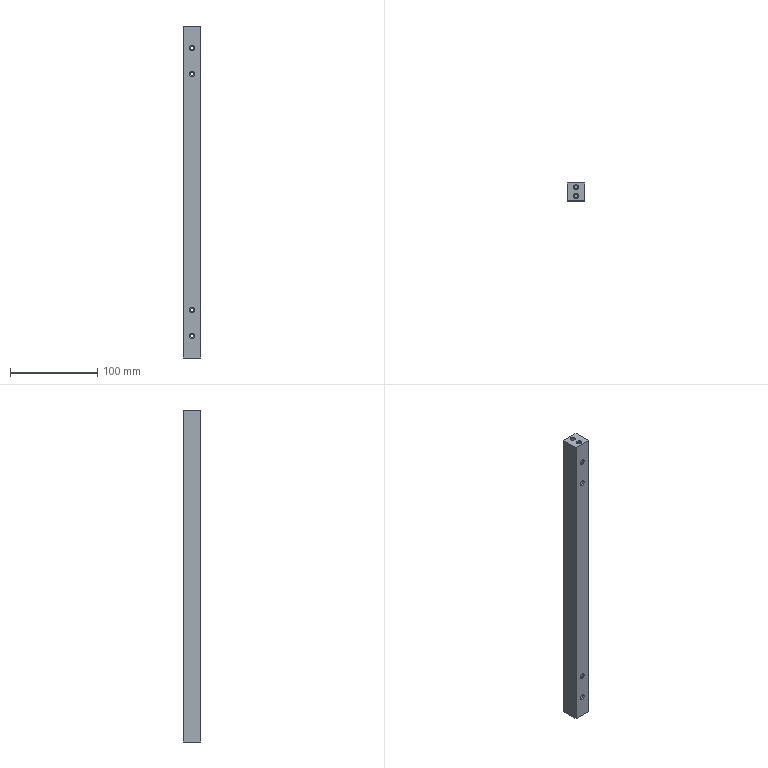Part | STEP file | Support rod 2 | 1 solid | 50 faces | box 20 x 20 x 380 mm | volume 150404 mm3 | cone 24 | cylinder 16 | plane 10 | commonest cylinder face diameters 4 x16
STEP:
#1=CARTESIAN_POINT('',(-2.853,-6.276,1.));
#2=VERTEX_POINT('',#1);
#3=CARTESIAN_POINT('',(-6.853,-6.276,1.));
#4=VERTEX_POINT('',#3);
#5=CARTESIAN_POINT('',(-4.853,-6.276,1.));
#6=DIRECTION('',(0.,0.,-1.));
#7=DIRECTION('',(-1.,0.,0.));
#8=AXIS2_PLACEMENT_3D('',#5,#6,#7);
#9=CIRCLE('',#8,2.);
#10=EDGE_CURVE('',#2,#4,#9,.T.);
#11=ORIENTED_EDGE('',*,*,#10,.F.);
#12=CARTESIAN_POINT('',(-1.853,-6.276,0.));
#13=VERTEX_POINT('',#12);
#14=CARTESIAN_POINT('',(-1.853,-6.276,0.));
#15=DIRECTION('',(0.7071,0.,-0.7071));
#16=VECTOR('',#15,1000.);
#17=LINE('',#14,#16);
#18=EDGE_CURVE('',#2,#13,#17,.T.);
#19=ORIENTED_EDGE('',*,*,#18,.T.);
#20=CARTESIAN_POINT('',(-7.853,-6.276,0.));
#21=VERTEX_POINT('',#20);
#22=CARTESIAN_POINT('',(-4.853,-6.276,0.));
#23=DIRECTION('',(0.,0.,-1.));
#24=DIRECTION('',(-1.,0.,0.));
#25=AXIS2_PLACEMENT_3D('',#22,#23,#24);
#26=CIRCLE('',#25,3.);
#27=EDGE_CURVE('',#13,#21,#26,.T.);
#28=ORIENTED_EDGE('',*,*,#27,.T.);
#29=CARTESIAN_POINT('',(-7.853,-6.276,0.));
#30=DIRECTION('',(-0.7071,0.,-0.7071));
#31=VECTOR('',#30,1000.);
#32=LINE('',#29,#31);
#33=EDGE_CURVE('',#4,#21,#32,.T.);
#34=ORIENTED_EDGE('',*,*,#33,.F.);
#35=EDGE_LOOP('',(#11,#19,#28,#34));
#36=FACE_OUTER_BOUND('',#35,.T.);
#37=CARTESIAN_POINT('',(-4.853,-6.276,0.));
#38=DIRECTION('',(0.,0.,-1.));
#39=DIRECTION('',(-1.,0.,0.));
#40=AXIS2_PLACEMENT_3D('',#37,#38,#39);
#41=CONICAL_SURFACE('',#40,3.,0.7854);
#42=ADVANCED_FACE('',(#36),#41,.F.);
#43=CARTESIAN_POINT('',(-2.853,-16.276,1.));
#44=VERTEX_POINT('',#43);
#45=CARTESIAN_POINT('',(-6.853,-16.276,1.));
#46=VERTEX_POINT('',#45);
#47=CARTESIAN_POINT('',(-4.853,-16.276,1.));
#48=DIRECTION('',(0.,0.,-1.));
#49=DIRECTION('',(-1.,0.,0.));
#50=AXIS2_PLACEMENT_3D('',#47,#48,#49);
#51=CIRCLE('',#50,2.);
#52=EDGE_CURVE('',#44,#46,#51,.T.);
#53=ORIENTED_EDGE('',*,*,#52,.F.);
#54=CARTESIAN_POINT('',(-1.853,-16.276,0.));
#55=VERTEX_POINT('',#54);
#56=CARTESIAN_POINT('',(-1.853,-16.276,0.));
#57=DIRECTION('',(0.7071,0.,-0.7071));
#58=VECTOR('',#57,1000.);
#59=LINE('',#56,#58);
#60=EDGE_CURVE('',#44,#55,#59,.T.);
#61=ORIENTED_EDGE('',*,*,#60,.T.);
#62=CARTESIAN_POINT('',(-7.853,-16.276,0.));
#63=VERTEX_POINT('',#62);
#64=CARTESIAN_POINT('',(-4.853,-16.276,0.));
#65=DIRECTION('',(0.,0.,-1.));
#66=DIRECTION('',(-1.,0.,0.));
#67=AXIS2_PLACEMENT_3D('',#64,#65,#66);
#68=CIRCLE('',#67,3.);
#69=EDGE_CURVE('',#55,#63,#68,.T.);
#70=ORIENTED_EDGE('',*,*,#69,.T.);
#71=CARTESIAN_POINT('',(-7.853,-16.276,0.));
#72=DIRECTION('',(-0.7071,0.,-0.7071));
#73=VECTOR('',#72,1000.);
#74=LINE('',#71,#73);
#75=EDGE_CURVE('',#46,#63,#74,.T.);
#76=ORIENTED_EDGE('',*,*,#75,.F.);
#77=EDGE_LOOP('',(#53,#61,#70,#76));
#78=FACE_OUTER_BOUND('',#77,.T.);
#79=CARTESIAN_POINT('',(-4.853,-16.276,0.));
#80=DIRECTION('',(0.,0.,-1.));
#81=DIRECTION('',(-1.,0.,0.));
#82=AXIS2_PLACEMENT_3D('',#79,#80,#81);
#83=CONICAL_SURFACE('',#82,3.,0.7854);
#84=ADVANCED_FACE('',(#78),#83,.F.);
#85=CARTESIAN_POINT('',(-4.853,-2.276,23.));
#86=VERTEX_POINT('',#85);
#87=CARTESIAN_POINT('',(-4.853,-2.276,27.));
#88=VERTEX_POINT('',#87);
#89=CARTESIAN_POINT('',(-4.853,-2.276,25.));
#90=DIRECTION('',(0.,1.,0.));
#91=DIRECTION('',(0.,0.,1.));
#92=AXIS2_PLACEMENT_3D('',#89,#90,#91);
#93=CIRCLE('',#92,2.);
#94=EDGE_CURVE('',#86,#88,#93,.T.);
#95=ORIENTED_EDGE('',*,*,#94,.F.);
#96=CARTESIAN_POINT('',(-4.853,-1.276,22.));
#97=VERTEX_POINT('',#96);
#98=CARTESIAN_POINT('',(-4.853,-1.276,22.));
#99=DIRECTION('',(0.,0.7071,-0.7071));
#100=VECTOR('',#99,1000.);
#101=LINE('',#98,#100);
#102=EDGE_CURVE('',#86,#97,#101,.T.);
#103=ORIENTED_EDGE('',*,*,#102,.T.);
#104=CARTESIAN_POINT('',(-4.853,-1.276,28.));
#105=VERTEX_POINT('',#104);
#106=CARTESIAN_POINT('',(-4.853,-1.276,25.));
#107=DIRECTION('',(0.,1.,0.));
#108=DIRECTION('',(0.,0.,1.));
#109=AXIS2_PLACEMENT_3D('',#106,#107,#108);
#110=CIRCLE('',#109,3.);
#111=EDGE_CURVE('',#97,#105,#110,.T.);
#112=ORIENTED_EDGE('',*,*,#111,.T.);
#113=CARTESIAN_POINT('',(-4.853,-1.276,28.));
#114=DIRECTION('',(0.,0.7071,0.7071));
#115=VECTOR('',#114,1000.);
#116=LINE('',#113,#115);
#117=EDGE_CURVE('',#88,#105,#116,.T.);
#118=ORIENTED_EDGE('',*,*,#117,.F.);
#119=EDGE_LOOP('',(#95,#103,#112,#118));
#120=FACE_OUTER_BOUND('',#119,.T.);
#121=CARTESIAN_POINT('',(-4.853,-1.276,25.));
#122=DIRECTION('',(0.,1.,0.));
#123=DIRECTION('',(0.,0.,1.));
#124=AXIS2_PLACEMENT_3D('',#121,#122,#123);
#125=CONICAL_SURFACE('',#124,3.,0.7854);
#126=ADVANCED_FACE('',(#120),#125,.F.);
#127=CARTESIAN_POINT('',(-4.853,-2.276,53.));
#128=VERTEX_POINT('',#127);
#129=CARTESIAN_POINT('',(-4.853,-2.276,57.));
#130=VERTEX_POINT('',#129);
#131=CARTESIAN_POINT('',(-4.853,-2.276,55.));
#132=DIRECTION('',(0.,1.,0.));
#133=DIRECTION('',(0.,0.,1.));
#134=AXIS2_PLACEMENT_3D('',#131,#132,#133);
#135=CIRCLE('',#134,2.);
#136=EDGE_CURVE('',#128,#130,#135,.T.);
#137=ORIENTED_EDGE('',*,*,#136,.F.);
#138=CARTESIAN_POINT('',(-4.853,-1.276,52.));
#139=VERTEX_POINT('',#138);
#140=CARTESIAN_POINT('',(-4.853,-1.276,52.));
#141=DIRECTION('',(0.,0.7071,-0.7071));
#142=VECTOR('',#141,1000.);
#143=LINE('',#140,#142);
#144=EDGE_CURVE('',#128,#139,#143,.T.);
#145=ORIENTED_EDGE('',*,*,#144,.T.);
#146=CARTESIAN_POINT('',(-4.853,-1.276,58.));
#147=VERTEX_POINT('',#146);
#148=CARTESIAN_POINT('',(-4.853,-1.276,55.));
#149=DIRECTION('',(0.,1.,0.));
#150=DIRECTION('',(0.,0.,1.));
#151=AXIS2_PLACEMENT_3D('',#148,#149,#150);
#152=CIRCLE('',#151,3.);
#153=EDGE_CURVE('',#139,#147,#152,.T.);
#154=ORIENTED_EDGE('',*,*,#153,.T.);
#155=CARTESIAN_POINT('',(-4.853,-1.276,58.));
#156=DIRECTION('',(0.,0.7071,0.7071));
#157=VECTOR('',#156,1000.);
#158=LINE('',#155,#157);
#159=EDGE_CURVE('',#130,#147,#158,.T.);
#160=ORIENTED_EDGE('',*,*,#159,.F.);
#161=EDGE_LOOP('',(#137,#145,#154,#160));
#162=FACE_OUTER_BOUND('',#161,.T.);
#163=CARTESIAN_POINT('',(-4.853,-1.276,55.));
#164=DIRECTION('',(0.,1.,0.));
#165=DIRECTION('',(0.,0.,1.));
#166=AXIS2_PLACEMENT_3D('',#163,#164,#165);
#167=CONICAL_SURFACE('',#166,3.,0.7854);
#168=ADVANCED_FACE('',(#162),#167,.F.);
#169=CARTESIAN_POINT('',(-4.853,-2.276,323.));
#170=VERTEX_POINT('',#169);
#171=CARTESIAN_POINT('',(-4.853,-2.276,327.));
#172=VERTEX_POINT('',#171);
#173=CARTESIAN_POINT('',(-4.853,-2.276,325.));
#174=DIRECTION('',(0.,1.,0.));
#175=DIRECTION('',(0.,0.,1.));
#176=AXIS2_PLACEMENT_3D('',#173,#174,#175);
#177=CIRCLE('',#176,2.);
#178=EDGE_CURVE('',#170,#172,#177,.T.);
#179=ORIENTED_EDGE('',*,*,#178,.F.);
#180=CARTESIAN_POINT('',(-4.853,-1.276,322.));
#181=VERTEX_POINT('',#180);
#182=CARTESIAN_POINT('',(-4.853,-1.276,322.));
#183=DIRECTION('',(0.,0.7071,-0.7071));
#184=VECTOR('',#183,1000.);
#185=LINE('',#182,#184);
#186=EDGE_CURVE('',#170,#181,#185,.T.);
#187=ORIENTED_EDGE('',*,*,#186,.T.);
#188=CARTESIAN_POINT('',(-4.853,-1.276,328.));
#189=VERTEX_POINT('',#188);
#190=CARTESIAN_POINT('',(-4.853,-1.276,325.));
#191=DIRECTION('',(0.,1.,0.));
#192=DIRECTION('',(0.,0.,1.));
#193=AXIS2_PLACEMENT_3D('',#190,#191,#192);
#194=CIRCLE('',#193,3.);
#195=EDGE_CURVE('',#181,#189,#194,.T.);
#196=ORIENTED_EDGE('',*,*,#195,.T.);
#197=CARTESIAN_POINT('',(-4.853,-1.276,328.));
#198=DIRECTION('',(0.,0.7071,0.7071));
#199=VECTOR('',#198,1000.);
#200=LINE('',#197,#199);
#201=EDGE_CURVE('',#172,#189,#200,.T.);
#202=ORIENTED_EDGE('',*,*,#201,.F.);
#203=EDGE_LOOP('',(#179,#187,#196,#202));
#204=FACE_OUTER_BOUND('',#203,.T.);
#205=CARTESIAN_POINT('',(-4.853,-1.276,325.));
#206=DIRECTION('',(0.,1.,0.));
#207=DIRECTION('',(0.,0.,1.));
#208=AXIS2_PLACEMENT_3D('',#205,#206,#207);
#209=CONICAL_SURFACE('',#208,3.,0.7854);
#210=ADVANCED_FACE('',(#204),#209,.F.);
#211=CARTESIAN_POINT('',(-4.853,-2.276,353.));
#212=VERTEX_POINT('',#211);
#213=CARTESIAN_POINT('',(-4.853,-2.276,357.));
#214=VERTEX_POINT('',#213);
#215=CARTESIAN_POINT('',(-4.853,-2.276,355.));
#216=DIRECTION('',(0.,1.,0.));
#217=DIRECTION('',(0.,0.,1.));
#218=AXIS2_PLACEMENT_3D('',#215,#216,#217);
#219=CIRCLE('',#218,2.);
#220=EDGE_CURVE('',#212,#214,#219,.T.);
#221=ORIENTED_EDGE('',*,*,#220,.F.);
#222=CARTESIAN_POINT('',(-4.853,-1.276,352.));
#223=VERTEX_POINT('',#222);
#224=CARTESIAN_POINT('',(-4.853,-1.276,352.));
#225=DIRECTION('',(0.,0.7071,-0.7071));
#226=VECTOR('',#225,1000.);
#227=LINE('',#224,#226);
#228=EDGE_CURVE('',#212,#223,#227,.T.);
#229=ORIENTED_EDGE('',*,*,#228,.T.);
#230=CARTESIAN_POINT('',(-4.853,-1.276,358.));
#231=VERTEX_POINT('',#230);
#232=CARTESIAN_POINT('',(-4.853,-1.276,355.));
#233=DIRECTION('',(0.,1.,0.));
#234=DIRECTION('',(0.,0.,1.));
#235=AXIS2_PLACEMENT_3D('',#232,#233,#234);
#236=CIRCLE('',#235,3.);
#237=EDGE_CURVE('',#223,#231,#236,.T.);
#238=ORIENTED_EDGE('',*,*,#237,.T.);
#239=CARTESIAN_POINT('',(-4.853,-1.276,358.));
#240=DIRECTION('',(0.,0.7071,0.7071));
#241=VECTOR('',#240,1000.);
#242=LINE('',#239,#241);
#243=EDGE_CURVE('',#214,#231,#242,.T.);
#244=ORIENTED_EDGE('',*,*,#243,.F.);
#245=EDGE_LOOP('',(#221,#229,#238,#244));
#246=FACE_OUTER_BOUND('',#245,.T.);
#247=CARTESIAN_POINT('',(-4.853,-1.276,355.));
#248=DIRECTION('',(0.,1.,0.));
#249=DIRECTION('',(0.,0.,1.));
#250=AXIS2_PLACEMENT_3D('',#247,#248,#249);
#251=CONICAL_SURFACE('',#250,3.,0.7854);
#252=ADVANCED_FACE('',(#246),#251,.F.);
#253=CARTESIAN_POINT('',(-4.853,-4.276,379.));
#254=VERTEX_POINT('',#253);
#255=CARTESIAN_POINT('',(-6.853,-6.276,379.));
#256=VERTEX_POINT('',#255);
#257=CARTESIAN_POINT('',(-4.853,-6.276,379.));
#258=DIRECTION('',(0.,0.,1.));
#259=DIRECTION('',(1.,0.,0.));
#260=AXIS2_PLACEMENT_3D('',#257,#258,#259);
#261=CIRCLE('',#260,2.);
#262=EDGE_CURVE('',#254,#256,#261,.T.);
#263=ORIENTED_EDGE('',*,*,#262,.F.);
#264=CARTESIAN_POINT('',(-4.853,-3.276,380.));
#265=VERTEX_POINT('',#264);
#266=CARTESIAN_POINT('',(-4.853,-3.276,380.));
#267=DIRECTION('',(0.,0.7071,0.7071));
#268=VECTOR('',#267,1000.);
#269=LINE('',#266,#268);
#270=EDGE_CURVE('',#254,#265,#269,.T.);
#271=ORIENTED_EDGE('',*,*,#270,.T.);
#272=CARTESIAN_POINT('',(-4.853,-9.276,380.));
#273=VERTEX_POINT('',#272);
#274=CARTESIAN_POINT('',(-4.853,-6.276,380.));
#275=DIRECTION('',(0.,0.,-1.));
#276=DIRECTION('',(0.,-1.,0.));
#277=AXIS2_PLACEMENT_3D('',#274,#275,#276);
#278=CIRCLE('',#277,3.);
#279=EDGE_CURVE('',#273,#265,#278,.T.);
#280=ORIENTED_EDGE('',*,*,#279,.F.);
#281=CARTESIAN_POINT('',(-4.853,-8.276,379.));
#282=VERTEX_POINT('',#281);
#283=CARTESIAN_POINT('',(-4.853,-9.276,380.));
#284=DIRECTION('',(0.,-0.7071,0.7071));
#285=VECTOR('',#284,1000.);
#286=LINE('',#283,#285);
#287=EDGE_CURVE('',#282,#273,#286,.T.);
#288=ORIENTED_EDGE('',*,*,#287,.F.);
#289=CARTESIAN_POINT('',(-4.853,-6.276,379.));
#290=DIRECTION('',(0.,0.,1.));
#291=DIRECTION('',(1.,0.,0.));
#292=AXIS2_PLACEMENT_3D('',#289,#290,#291);
#293=CIRCLE('',#292,2.);
#294=EDGE_CURVE('',#256,#282,#293,.T.);
#295=ORIENTED_EDGE('',*,*,#294,.F.);
#296=EDGE_LOOP('',(#263,#271,#280,#288,#295));
#297=FACE_OUTER_BOUND('',#296,.T.);
#298=CARTESIAN_POINT('',(-4.853,-6.276,380.));
#299=DIRECTION('',(0.,0.,1.));
#300=DIRECTION('',(0.,-1.,0.));
#301=AXIS2_PLACEMENT_3D('',#298,#299,#300);
#302=CONICAL_SURFACE('',#301,3.,0.7854);
#303=ADVANCED_FACE('',(#297),#302,.F.);
#304=CARTESIAN_POINT('',(-6.853,-16.276,379.));
#305=VERTEX_POINT('',#304);
#306=CARTESIAN_POINT('',(-2.853,-16.276,379.));
#307=VERTEX_POINT('',#306);
#308=CARTESIAN_POINT('',(-4.853,-16.276,379.));
#309=DIRECTION('',(0.,0.,1.));
#310=DIRECTION('',(1.,0.,0.));
#311=AXIS2_PLACEMENT_3D('',#308,#309,#310);
#312=CIRCLE('',#311,2.);
#313=EDGE_CURVE('',#305,#307,#312,.T.);
#314=ORIENTED_EDGE('',*,*,#313,.F.);
#315=CARTESIAN_POINT('',(-7.853,-16.276,380.));
#316=VERTEX_POINT('',#315);
#317=CARTESIAN_POINT('',(-7.853,-16.276,380.));
#318=DIRECTION('',(-0.7071,0.,0.7071));
#319=VECTOR('',#318,1000.);
#320=LINE('',#317,#319);
#321=EDGE_CURVE('',#305,#316,#320,.T.);
#322=ORIENTED_EDGE('',*,*,#321,.T.);
#323=CARTESIAN_POINT('',(-1.853,-16.276,380.));
#324=VERTEX_POINT('',#323);
#325=CARTESIAN_POINT('',(-4.853,-16.276,380.));
#326=DIRECTION('',(0.,0.,-1.));
#327=DIRECTION('',(1.,0.,0.));
#328=AXIS2_PLACEMENT_3D('',#325,#326,#327);
#329=CIRCLE('',#328,3.);
#330=EDGE_CURVE('',#324,#316,#329,.T.);
#331=ORIENTED_EDGE('',*,*,#330,.F.);
#332=CARTESIAN_POINT('',(-1.853,-16.276,380.));
#333=DIRECTION('',(0.7071,0.,0.7071));
#334=VECTOR('',#333,1000.);
#335=LINE('',#332,#334);
#336=EDGE_CURVE('',#307,#324,#335,.T.);
#337=ORIENTED_EDGE('',*,*,#336,.F.);
#338=EDGE_LOOP('',(#314,#322,#331,#337));
#339=FACE_OUTER_BOUND('',#338,.T.);
#340=CARTESIAN_POINT('',(-4.853,-16.276,380.));
#341=DIRECTION('',(0.,0.,1.));
#342=DIRECTION('',(1.,0.,0.));
#343=AXIS2_PLACEMENT_3D('',#340,#341,#342);
#344=CONICAL_SURFACE('',#343,3.,0.7854);
#345=ADVANCED_FACE('',(#339),#344,.F.);
#346=CARTESIAN_POINT('',(-4.853,-20.276,27.));
#347=VERTEX_POINT('',#346);
#348=CARTESIAN_POINT('',(-4.853,-20.276,23.));
#349=VERTEX_POINT('',#348);
#350=CARTESIAN_POINT('',(-4.853,-20.276,25.));
#351=DIRECTION('',(0.,-1.,0.));
#352=DIRECTION('',(0.,0.,-1.));
#353=AXIS2_PLACEMENT_3D('',#350,#351,#352);
#354=CIRCLE('',#353,2.);
#355=EDGE_CURVE('',#347,#349,#354,.T.);
#356=ORIENTED_EDGE('',*,*,#355,.F.);
#357=CARTESIAN_POINT('',(-4.853,-21.276,28.));
#358=VERTEX_POINT('',#357);
#359=CARTESIAN_POINT('',(-4.853,-21.276,28.));
#360=DIRECTION('',(0.,-0.7071,0.7071));
#361=VECTOR('',#360,1000.);
#362=LINE('',#359,#361);
#363=EDGE_CURVE('',#347,#358,#362,.T.);
#364=ORIENTED_EDGE('',*,*,#363,.T.);
#365=CARTESIAN_POINT('',(-4.853,-21.276,22.));
#366=VERTEX_POINT('',#365);
#367=CARTESIAN_POINT('',(-4.853,-21.276,25.));
#368=DIRECTION('',(0.,-1.,0.));
#369=DIRECTION('',(0.,0.,-1.));
#370=AXIS2_PLACEMENT_3D('',#367,#368,#369);
#371=CIRCLE('',#370,3.);
#372=EDGE_CURVE('',#358,#366,#371,.T.);
#373=ORIENTED_EDGE('',*,*,#372,.T.);
#374=CARTESIAN_POINT('',(-4.853,-21.276,22.));
#375=DIRECTION('',(0.,-0.7071,-0.7071));
#376=VECTOR('',#375,1000.);
#377=LINE('',#374,#376);
#378=EDGE_CURVE('',#349,#366,#377,.T.);
#379=ORIENTED_EDGE('',*,*,#378,.F.);
#380=EDGE_LOOP('',(#356,#364,#373,#379));
#381=FACE_OUTER_BOUND('',#380,.T.);
#382=CARTESIAN_POINT('',(-4.853,-21.276,25.));
#383=DIRECTION('',(0.,-1.,0.));
#384=DIRECTION('',(0.,0.,-1.));
#385=AXIS2_PLACEMENT_3D('',#382,#383,#384);
#386=CONICAL_SURFACE('',#385,3.,0.7854);
#387=ADVANCED_FACE('',(#381),#386,.F.);
#388=CARTESIAN_POINT('',(-4.853,-20.276,57.));
#389=VERTEX_POINT('',#388);
#390=CARTESIAN_POINT('',(-4.853,-20.276,53.));
#391=VERTEX_POINT('',#390);
#392=CARTESIAN_POINT('',(-4.853,-20.276,55.));
#393=DIRECTION('',(0.,-1.,0.));
#394=DIRECTION('',(0.,0.,-1.));
#395=AXIS2_PLACEMENT_3D('',#392,#393,#394);
#396=CIRCLE('',#395,2.);
#397=EDGE_CURVE('',#389,#391,#396,.T.);
#398=ORIENTED_EDGE('',*,*,#397,.F.);
#399=CARTESIAN_POINT('',(-4.853,-21.276,58.));
#400=VERTEX_POINT('',#399);
#401=CARTESIAN_POINT('',(-4.853,-21.276,58.));
#402=DIRECTION('',(0.,-0.7071,0.7071));
#403=VECTOR('',#402,1000.);
#404=LINE('',#401,#403);
#405=EDGE_CURVE('',#389,#400,#404,.T.);
#406=ORIENTED_EDGE('',*,*,#405,.T.);
#407=CARTESIAN_POINT('',(-4.853,-21.276,52.));
#408=VERTEX_POINT('',#407);
#409=CARTESIAN_POINT('',(-4.853,-21.276,55.));
#410=DIRECTION('',(0.,-1.,0.));
#411=DIRECTION('',(0.,0.,-1.));
#412=AXIS2_PLACEMENT_3D('',#409,#410,#411);
#413=CIRCLE('',#412,3.);
#414=EDGE_CURVE('',#400,#408,#413,.T.);
#415=ORIENTED_EDGE('',*,*,#414,.T.);
#416=CARTESIAN_POINT('',(-4.853,-21.276,52.));
#417=DIRECTION('',(0.,-0.7071,-0.7071));
#418=VECTOR('',#417,1000.);
#419=LINE('',#416,#418);
#420=EDGE_CURVE('',#391,#408,#419,.T.);
#421=ORIENTED_EDGE('',*,*,#420,.F.);
#422=EDGE_LOOP('',(#398,#406,#415,#421));
#423=FACE_OUTER_BOUND('',#422,.T.);
#424=CARTESIAN_POINT('',(-4.853,-21.276,55.));
#425=DIRECTION('',(0.,-1.,0.));
#426=DIRECTION('',(0.,0.,-1.));
#427=AXIS2_PLACEMENT_3D('',#424,#425,#426);
#428=CONICAL_SURFACE('',#427,3.,0.7854);
#429=ADVANCED_FACE('',(#423),#428,.F.);
#430=CARTESIAN_POINT('',(-4.853,-20.276,327.));
#431=VERTEX_POINT('',#430);
#432=CARTESIAN_POINT('',(-4.853,-20.276,323.));
#433=VERTEX_POINT('',#432);
#434=CARTESIAN_POINT('',(-4.853,-20.276,325.));
#435=DIRECTION('',(0.,-1.,0.));
#436=DIRECTION('',(0.,0.,-1.));
#437=AXIS2_PLACEMENT_3D('',#434,#435,#436);
#438=CIRCLE('',#437,2.);
#439=EDGE_CURVE('',#431,#433,#438,.T.);
#440=ORIENTED_EDGE('',*,*,#439,.F.);
#441=CARTESIAN_POINT('',(-4.853,-21.276,328.));
#442=VERTEX_POINT('',#441);
#443=CARTESIAN_POINT('',(-4.853,-21.276,328.));
#444=DIRECTION('',(0.,-0.7071,0.7071));
#445=VECTOR('',#444,1000.);
#446=LINE('',#443,#445);
#447=EDGE_CURVE('',#431,#442,#446,.T.);
#448=ORIENTED_EDGE('',*,*,#447,.T.);
#449=CARTESIAN_POINT('',(-4.853,-21.276,322.));
#450=VERTEX_POINT('',#449);
#451=CARTESIAN_POINT('',(-4.853,-21.276,325.));
#452=DIRECTION('',(0.,-1.,0.));
#453=DIRECTION('',(0.,0.,-1.));
#454=AXIS2_PLACEMENT_3D('',#451,#452,#453);
#455=CIRCLE('',#454,3.);
#456=EDGE_CURVE('',#442,#450,#455,.T.);
#457=ORIENTED_EDGE('',*,*,#456,.T.);
#458=CARTESIAN_POINT('',(-4.853,-21.276,322.));
#459=DIRECTION('',(0.,-0.7071,-0.7071));
#460=VECTOR('',#459,1000.);
#461=LINE('',#458,#460);
#462=EDGE_CURVE('',#433,#450,#461,.T.);
#463=ORIENTED_EDGE('',*,*,#462,.F.);
#464=EDGE_LOOP('',(#440,#448,#457,#463));
#465=FACE_OUTER_BOUND('',#464,.T.);
#466=CARTESIAN_POINT('',(-4.853,-21.276,325.));
#467=DIRECTION('',(0.,-1.,0.));
#468=DIRECTION('',(0.,0.,-1.));
#469=AXIS2_PLACEMENT_3D('',#466,#467,#468);
#470=CONICAL_SURFACE('',#469,3.,0.7854);
#471=ADVANCED_FACE('',(#465),#470,.F.);
#472=CARTESIAN_POINT('',(-4.853,-20.276,357.));
#473=VERTEX_POINT('',#472);
#474=CARTESIAN_POINT('',(-4.853,-20.276,353.));
#475=VERTEX_POINT('',#474);
#476=CARTESIAN_POINT('',(-4.853,-20.276,355.));
#477=DIRECTION('',(0.,-1.,0.));
#478=DIRECTION('',(0.,0.,-1.));
#479=AXIS2_PLACEMENT_3D('',#476,#477,#478);
#480=CIRCLE('',#479,2.);
#481=EDGE_CURVE('',#473,#475,#480,.T.);
#482=ORIENTED_EDGE('',*,*,#481,.F.);
#483=CARTESIAN_POINT('',(-4.853,-21.276,358.));
#484=VERTEX_POINT('',#483);
#485=CARTESIAN_POINT('',(-4.853,-21.276,358.));
#486=DIRECTION('',(0.,-0.7071,0.7071));
#487=VECTOR('',#486,1000.);
#488=LINE('',#485,#487);
#489=EDGE_CURVE('',#473,#484,#488,.T.);
#490=ORIENTED_EDGE('',*,*,#489,.T.);
#491=CARTESIAN_POINT('',(-4.853,-21.276,352.));
#492=VERTEX_POINT('',#491);
#493=CARTESIAN_POINT('',(-4.853,-21.276,355.));
#494=DIRECTION('',(0.,-1.,0.));
#495=DIRECTION('',(0.,0.,-1.));
#496=AXIS2_PLACEMENT_3D('',#493,#494,#495);
#497=CIRCLE('',#496,3.);
#498=EDGE_CURVE('',#484,#492,#497,.T.);
#499=ORIENTED_EDGE('',*,*,#498,.T.);
#500=CARTESIAN_POINT('',(-4.853,-21.276,352.));
#501=DIRECTION('',(0.,-0.7071,-0.7071));
#502=VECTOR('',#501,1000.);
#503=LINE('',#500,#502);
#504=EDGE_CURVE('',#475,#492,#503,.T.);
#505=ORIENTED_EDGE('',*,*,#504,.F.);
#506=EDGE_LOOP('',(#482,#490,#499,#505));
#507=FACE_OUTER_BOUND('',#506,.T.);
#508=CARTESIAN_POINT('',(-4.853,-21.276,355.));
#509=DIRECTION('',(0.,-1.,0.));
#510=DIRECTION('',(0.,0.,-1.));
#511=AXIS2_PLACEMENT_3D('',#508,#509,#510);
#512=CONICAL_SURFACE('',#511,3.,0.7854);
#513=ADVANCED_FACE('',(#507),#512,.F.);
#514=CARTESIAN_POINT('',(-2.853,-6.276,10.));
#515=VERTEX_POINT('',#514);
#516=CARTESIAN_POINT('',(-6.853,-6.276,10.));
#517=VERTEX_POINT('',#516);
#518=CARTESIAN_POINT('',(-4.853,-6.276,10.));
#519=DIRECTION('',(0.,0.,-1.));
#520=DIRECTION('',(-1.,0.,0.));
#521=AXIS2_PLACEMENT_3D('',#518,#519,#520);
#522=CIRCLE('',#521,2.);
#523=EDGE_CURVE('',#515,#517,#522,.T.);
#524=ORIENTED_EDGE('',*,*,#523,.F.);
#525=CARTESIAN_POINT('',(-2.853,-6.276,10.));
#526=DIRECTION('',(0.,0.,-1.));
#527=VECTOR('',#526,1000.);
#528=LINE('',#525,#527);
#529=EDGE_CURVE('',#515,#2,#528,.T.);
#530=ORIENTED_EDGE('',*,*,#529,.T.);
#531=ORIENTED_EDGE('',*,*,#10,.T.);
#532=CARTESIAN_POINT('',(-6.853,-6.276,10.));
#533=DIRECTION('',(0.,0.,-1.));
#534=VECTOR('',#533,1000.);
#535=LINE('',#532,#534);
#536=EDGE_CURVE('',#517,#4,#535,.T.);
#537=ORIENTED_EDGE('',*,*,#536,.F.);
#538=EDGE_LOOP('',(#524,#530,#531,#537));
#539=FACE_OUTER_BOUND('',#538,.T.);
#540=CARTESIAN_POINT('',(-4.853,-6.276,10.));
#541=DIRECTION('',(0.,0.,-1.));
#542=DIRECTION('',(-1.,0.,0.));
#543=AXIS2_PLACEMENT_3D('',#540,#541,#542);
#544=CYLINDRICAL_SURFACE('',#543,2.);
#545=ADVANCED_FACE('',(#539),#544,.F.);
#546=CARTESIAN_POINT('',(-2.853,-16.276,10.));
#547=VERTEX_POINT('',#546);
#548=CARTESIAN_POINT('',(-6.853,-16.276,10.));
#549=VERTEX_POINT('',#548);
#550=CARTESIAN_POINT('',(-4.853,-16.276,10.));
#551=DIRECTION('',(0.,0.,-1.));
#552=DIRECTION('',(-1.,0.,0.));
#553=AXIS2_PLACEMENT_3D('',#550,#551,#552);
#554=CIRCLE('',#553,2.);
#555=EDGE_CURVE('',#547,#549,#554,.T.);
#556=ORIENTED_EDGE('',*,*,#555,.F.);
#557=CARTESIAN_POINT('',(-2.853,-16.276,10.));
#558=DIRECTION('',(0.,0.,-1.));
#559=VECTOR('',#558,1000.);
#560=LINE('',#557,#559);
#561=EDGE_CURVE('',#547,#44,#560,.T.);
#562=ORIENTED_EDGE('',*,*,#561,.T.);
#563=ORIENTED_EDGE('',*,*,#52,.T.);
#564=CARTESIAN_POINT('',(-6.853,-16.276,10.));
#565=DIRECTION('',(0.,0.,-1.));
#566=VECTOR('',#565,1000.);
#567=LINE('',#564,#566);
#568=EDGE_CURVE('',#549,#46,#567,.T.);
#569=ORIENTED_EDGE('',*,*,#568,.F.);
#570=EDGE_LOOP('',(#556,#562,#563,#569));
#571=FACE_OUTER_BOUND('',#570,.T.);
#572=CARTESIAN_POINT('',(-4.853,-16.276,10.));
#573=DIRECTION('',(0.,0.,-1.));
#574=DIRECTION('',(-1.,0.,0.));
#575=AXIS2_PLACEMENT_3D('',#572,#573,#574);
#576=CYLINDRICAL_SURFACE('',#575,2.);
#577=ADVANCED_FACE('',(#571),#576,.F.);
#578=ORIENTED_EDGE('',*,*,#355,.T.);
#579=CARTESIAN_POINT('',(-4.853,-21.276,23.));
#580=DIRECTION('',(0.,1.,0.));
#581=VECTOR('',#580,1000.);
#582=LINE('',#579,#581);
#583=EDGE_CURVE('',#349,#86,#582,.T.);
#584=ORIENTED_EDGE('',*,*,#583,.T.);
#585=ORIENTED_EDGE('',*,*,#94,.T.);
#586=CARTESIAN_POINT('',(-4.853,-21.276,27.));
#587=DIRECTION('',(0.,1.,0.));
#588=VECTOR('',#587,1000.);
#589=LINE('',#586,#588);
#590=EDGE_CURVE('',#347,#88,#589,.T.);
#591=ORIENTED_EDGE('',*,*,#590,.F.);
#592=EDGE_LOOP('',(#578,#584,#585,#591));
#593=FACE_OUTER_BOUND('',#592,.T.);
#594=CARTESIAN_POINT('',(-4.853,-21.276,25.));
#595=DIRECTION('',(0.,1.,0.));
#596=DIRECTION('',(0.,0.,1.));
#597=AXIS2_PLACEMENT_3D('',#594,#595,#596);
#598=CYLINDRICAL_SURFACE('',#597,2.);
#599=ADVANCED_FACE('',(#593),#598,.F.);
#600=ORIENTED_EDGE('',*,*,#397,.T.);
#601=CARTESIAN_POINT('',(-4.853,-21.276,53.));
#602=DIRECTION('',(0.,1.,0.));
#603=VECTOR('',#602,1000.);
#604=LINE('',#601,#603);
#605=EDGE_CURVE('',#391,#128,#604,.T.);
#606=ORIENTED_EDGE('',*,*,#605,.T.);
#607=ORIENTED_EDGE('',*,*,#136,.T.);
#608=CARTESIAN_POINT('',(-4.853,-21.276,57.));
#609=DIRECTION('',(0.,1.,0.));
#610=VECTOR('',#609,1000.);
#611=LINE('',#608,#610);
#612=EDGE_CURVE('',#389,#130,#611,.T.);
#613=ORIENTED_EDGE('',*,*,#612,.F.);
#614=EDGE_LOOP('',(#600,#606,#607,#613));
#615=FACE_OUTER_BOUND('',#614,.T.);
#616=CARTESIAN_POINT('',(-4.853,-21.276,55.));
#617=DIRECTION('',(0.,1.,0.));
#618=DIRECTION('',(0.,0.,1.));
#619=AXIS2_PLACEMENT_3D('',#616,#617,#618);
#620=CYLINDRICAL_SURFACE('',#619,2.);
#621=ADVANCED_FACE('',(#615),#620,.F.);
#622=ORIENTED_EDGE('',*,*,#439,.T.);
#623=CARTESIAN_POINT('',(-4.853,-21.276,323.));
#624=DIRECTION('',(0.,1.,0.));
#625=VECTOR('',#624,1000.);
#626=LINE('',#623,#625);
#627=EDGE_CURVE('',#433,#170,#626,.T.);
#628=ORIENTED_EDGE('',*,*,#627,.T.);
#629=ORIENTED_EDGE('',*,*,#178,.T.);
#630=CARTESIAN_POINT('',(-4.853,-21.276,327.));
#631=DIRECTION('',(0.,1.,0.));
#632=VECTOR('',#631,1000.);
#633=LINE('',#630,#632);
#634=EDGE_CURVE('',#431,#172,#633,.T.);
#635=ORIENTED_EDGE('',*,*,#634,.F.);
#636=EDGE_LOOP('',(#622,#628,#629,#635));
#637=FACE_OUTER_BOUND('',#636,.T.);
#638=CARTESIAN_POINT('',(-4.853,-21.276,325.));
#639=DIRECTION('',(0.,1.,0.));
#640=DIRECTION('',(0.,0.,1.));
#641=AXIS2_PLACEMENT_3D('',#638,#639,#640);
#642=CYLINDRICAL_SURFACE('',#641,2.);
#643=ADVANCED_FACE('',(#637),#642,.F.);
#644=ORIENTED_EDGE('',*,*,#481,.T.);
#645=CARTESIAN_POINT('',(-4.853,-21.276,353.));
#646=DIRECTION('',(0.,1.,0.));
#647=VECTOR('',#646,1000.);
#648=LINE('',#645,#647);
#649=EDGE_CURVE('',#475,#212,#648,.T.);
#650=ORIENTED_EDGE('',*,*,#649,.T.);
#651=ORIENTED_EDGE('',*,*,#220,.T.);
#652=CARTESIAN_POINT('',(-4.853,-21.276,357.));
#653=DIRECTION('',(0.,1.,0.));
#654=VECTOR('',#653,1000.);
#655=LINE('',#652,#654);
#656=EDGE_CURVE('',#473,#214,#655,.T.);
#657=ORIENTED_EDGE('',*,*,#656,.F.);
#658=EDGE_LOOP('',(#644,#650,#651,#657));
#659=FACE_OUTER_BOUND('',#658,.T.);
#660=CARTESIAN_POINT('',(-4.853,-21.276,355.));
#661=DIRECTION('',(0.,1.,0.));
#662=DIRECTION('',(0.,0.,1.));
#663=AXIS2_PLACEMENT_3D('',#660,#661,#662);
#664=CYLINDRICAL_SURFACE('',#663,2.);
#665=ADVANCED_FACE('',(#659),#664,.F.);
#666=CARTESIAN_POINT('',(-6.853,-6.276,370.));
#667=VERTEX_POINT('',#666);
#668=CARTESIAN_POINT('',(-2.853,-6.276,370.));
#669=VERTEX_POINT('',#668);
#670=CARTESIAN_POINT('',(-4.853,-6.276,370.));
#671=DIRECTION('',(0.,0.,1.));
#672=DIRECTION('',(1.,0.,0.));
#673=AXIS2_PLACEMENT_3D('',#670,#671,#672);
#674=CIRCLE('',#673,2.);
#675=EDGE_CURVE('',#667,#669,#674,.T.);
#676=ORIENTED_EDGE('',*,*,#675,.F.);
#677=CARTESIAN_POINT('',(-6.853,-6.276,370.));
#678=DIRECTION('',(0.,0.,1.));
#679=VECTOR('',#678,1000.);
#680=LINE('',#677,#679);
#681=EDGE_CURVE('',#667,#256,#680,.T.);
#682=ORIENTED_EDGE('',*,*,#681,.T.);
#683=ORIENTED_EDGE('',*,*,#294,.T.);
#684=CARTESIAN_POINT('',(-2.853,-6.276,379.));
#685=VERTEX_POINT('',#684);
#686=CARTESIAN_POINT('',(-4.853,-6.276,379.));
#687=DIRECTION('',(0.,0.,1.));
#688=DIRECTION('',(1.,0.,0.));
#689=AXIS2_PLACEMENT_3D('',#686,#687,#688);
#690=CIRCLE('',#689,2.);
#691=EDGE_CURVE('',#282,#685,#690,.T.);
#692=ORIENTED_EDGE('',*,*,#691,.T.);
#693=CARTESIAN_POINT('',(-2.853,-6.276,370.));
#694=DIRECTION('',(0.,0.,1.));
#695=VECTOR('',#694,1000.);
#696=LINE('',#693,#695);
#697=EDGE_CURVE('',#669,#685,#696,.T.);
#698=ORIENTED_EDGE('',*,*,#697,.F.);
#699=EDGE_LOOP('',(#676,#682,#683,#692,#698));
#700=FACE_OUTER_BOUND('',#699,.T.);
#701=CARTESIAN_POINT('',(-4.853,-6.276,370.));
#702=DIRECTION('',(0.,0.,1.));
#703=DIRECTION('',(1.,0.,0.));
#704=AXIS2_PLACEMENT_3D('',#701,#702,#703);
#705=CYLINDRICAL_SURFACE('',#704,2.);
#706=ADVANCED_FACE('',(#700),#705,.F.);
#707=CARTESIAN_POINT('',(-6.853,-16.276,370.));
#708=VERTEX_POINT('',#707);
#709=CARTESIAN_POINT('',(-2.853,-16.276,370.));
#710=VERTEX_POINT('',#709);
#711=CARTESIAN_POINT('',(-4.853,-16.276,370.));
#712=DIRECTION('',(0.,0.,1.));
#713=DIRECTION('',(1.,0.,0.));
#714=AXIS2_PLACEMENT_3D('',#711,#712,#713);
#715=CIRCLE('',#714,2.);
#716=EDGE_CURVE('',#708,#710,#715,.T.);
#717=ORIENTED_EDGE('',*,*,#716,.F.);
#718=CARTESIAN_POINT('',(-6.853,-16.276,370.));
#719=DIRECTION('',(0.,0.,1.));
#720=VECTOR('',#719,1000.);
#721=LINE('',#718,#720);
#722=EDGE_CURVE('',#708,#305,#721,.T.);
#723=ORIENTED_EDGE('',*,*,#722,.T.);
#724=ORIENTED_EDGE('',*,*,#313,.T.);
#725=CARTESIAN_POINT('',(-2.853,-16.276,370.));
#726=DIRECTION('',(0.,0.,1.));
#727=VECTOR('',#726,1000.);
#728=LINE('',#725,#727);
#729=EDGE_CURVE('',#710,#307,#728,.T.);
#730=ORIENTED_EDGE('',*,*,#729,.F.);
#731=EDGE_LOOP('',(#717,#723,#724,#730));
#732=FACE_OUTER_BOUND('',#731,.T.);
#733=CARTESIAN_POINT('',(-4.853,-16.276,370.));
#734=DIRECTION('',(0.,0.,1.));
#735=DIRECTION('',(1.,0.,0.));
#736=AXIS2_PLACEMENT_3D('',#733,#734,#735);
#737=CYLINDRICAL_SURFACE('',#736,2.);
#738=ADVANCED_FACE('',(#732),#737,.F.);
#739=CARTESIAN_POINT('',(5.147,-1.276,380.));
#740=VERTEX_POINT('',#739);
#741=CARTESIAN_POINT('',(5.147,-1.276,0.));
#742=VERTEX_POINT('',#741);
#743=CARTESIAN_POINT('',(5.147,-1.276,380.));
#744=DIRECTION('',(0.,0.,-1.));
#745=VECTOR('',#744,1000.);
#746=LINE('',#743,#745);
#747=EDGE_CURVE('',#740,#742,#746,.T.);
#748=ORIENTED_EDGE('',*,*,#747,.F.);
#749=CARTESIAN_POINT('',(5.147,-21.276,380.));
#750=VERTEX_POINT('',#749);
#751=CARTESIAN_POINT('',(5.147,-1.276,380.));
#752=DIRECTION('',(0.,1.,0.));
#753=VECTOR('',#752,1000.);
#754=LINE('',#751,#753);
#755=EDGE_CURVE('',#750,#740,#754,.T.);
#756=ORIENTED_EDGE('',*,*,#755,.F.);
#757=CARTESIAN_POINT('',(5.147,-21.276,0.));
#758=VERTEX_POINT('',#757);
#759=CARTESIAN_POINT('',(5.147,-21.276,380.));
#760=DIRECTION('',(0.,0.,1.));
#761=VECTOR('',#760,1000.);
#762=LINE('',#759,#761);
#763=EDGE_CURVE('',#758,#750,#762,.T.);
#764=ORIENTED_EDGE('',*,*,#763,.F.);
#765=CARTESIAN_POINT('',(5.147,-1.276,0.));
#766=DIRECTION('',(0.,-1.,0.));
#767=VECTOR('',#766,1000.);
#768=LINE('',#765,#767);
#769=EDGE_CURVE('',#742,#758,#768,.T.);
#770=ORIENTED_EDGE('',*,*,#769,.F.);
#771=EDGE_LOOP('',(#748,#756,#764,#770));
#772=FACE_OUTER_BOUND('',#771,.T.);
#773=CARTESIAN_POINT('',(5.147,-1.276,380.));
#774=DIRECTION('',(-1.,0.,0.));
#775=DIRECTION('',(0.,0.,1.));
#776=AXIS2_PLACEMENT_3D('',#773,#774,#775);
#777=PLANE('',#776);
#778=ADVANCED_FACE('',(#772),#777,.F.);
#779=CARTESIAN_POINT('',(-14.853,-1.276,0.));
#780=VERTEX_POINT('',#779);
#781=CARTESIAN_POINT('',(-14.853,-1.276,0.));
#782=DIRECTION('',(-1.,0.,0.));
#783=VECTOR('',#782,1000.);
#784=LINE('',#781,#783);
#785=EDGE_CURVE('',#742,#780,#784,.T.);
#786=ORIENTED_EDGE('',*,*,#785,.F.);
#787=ORIENTED_EDGE('',*,*,#769,.T.);
#788=CARTESIAN_POINT('',(-14.853,-21.276,0.));
#789=VERTEX_POINT('',#788);
#790=CARTESIAN_POINT('',(-14.853,-21.276,0.));
#791=DIRECTION('',(1.,0.,0.));
#792=VECTOR('',#791,1000.);
#793=LINE('',#790,#792);
#794=EDGE_CURVE('',#789,#758,#793,.T.);
#795=ORIENTED_EDGE('',*,*,#794,.F.);
#796=CARTESIAN_POINT('',(-14.853,-21.276,0.));
#797=DIRECTION('',(0.,-1.,0.));
#798=VECTOR('',#797,1000.);
#799=LINE('',#796,#798);
#800=EDGE_CURVE('',#780,#789,#799,.T.);
#801=ORIENTED_EDGE('',*,*,#800,.F.);
#802=EDGE_LOOP('',(#786,#787,#795,#801));
#803=FACE_OUTER_BOUND('',#802,.T.);
#804=CARTESIAN_POINT('',(-4.853,-6.276,0.));
#805=DIRECTION('',(0.,0.,-1.));
#806=DIRECTION('',(-1.,0.,0.));
#807=AXIS2_PLACEMENT_3D('',#804,#805,#806);
#808=CIRCLE('',#807,3.);
#809=EDGE_CURVE('',#21,#13,#808,.T.);
#810=ORIENTED_EDGE('',*,*,#809,.F.);
#811=ORIENTED_EDGE('',*,*,#27,.F.);
#812=EDGE_LOOP('',(#810,#811));
#813=FACE_BOUND('',#812,.T.);
#814=CARTESIAN_POINT('',(-4.853,-16.276,0.));
#815=DIRECTION('',(0.,0.,-1.));
#816=DIRECTION('',(-1.,0.,0.));
#817=AXIS2_PLACEMENT_3D('',#814,#815,#816);
#818=CIRCLE('',#817,3.);
#819=EDGE_CURVE('',#63,#55,#818,.T.);
#820=ORIENTED_EDGE('',*,*,#819,.F.);
#821=ORIENTED_EDGE('',*,*,#69,.F.);
#822=EDGE_LOOP('',(#820,#821));
#823=FACE_BOUND('',#822,.T.);
#824=CARTESIAN_POINT('',(-14.853,-21.276,0.));
#825=DIRECTION('',(0.,0.,1.));
#826=DIRECTION('',(1.,0.,0.));
#827=AXIS2_PLACEMENT_3D('',#824,#825,#826);
#828=PLANE('',#827);
#829=ADVANCED_FACE('',(#803,#813,#823),#828,.F.);
#830=CARTESIAN_POINT('',(-14.853,-1.276,380.));
#831=VERTEX_POINT('',#830);
#832=CARTESIAN_POINT('',(-14.853,-1.276,380.));
#833=DIRECTION('',(0.,0.,-1.));
#834=VECTOR('',#833,1000.);
#835=LINE('',#832,#834);
#836=EDGE_CURVE('',#831,#780,#835,.T.);
#837=ORIENTED_EDGE('',*,*,#836,.F.);
#838=CARTESIAN_POINT('',(-14.853,-1.276,380.));
#839=DIRECTION('',(-1.,0.,0.));
#840=VECTOR('',#839,1000.);
#841=LINE('',#838,#840);
#842=EDGE_CURVE('',#740,#831,#841,.T.);
#843=ORIENTED_EDGE('',*,*,#842,.F.);
#844=ORIENTED_EDGE('',*,*,#747,.T.);
#845=ORIENTED_EDGE('',*,*,#785,.T.);
#846=EDGE_LOOP('',(#837,#843,#844,#845));
#847=FACE_OUTER_BOUND('',#846,.T.);
#848=CARTESIAN_POINT('',(-4.853,-1.276,25.));
#849=DIRECTION('',(0.,1.,0.));
#850=DIRECTION('',(0.,0.,1.));
#851=AXIS2_PLACEMENT_3D('',#848,#849,#850);
#852=CIRCLE('',#851,3.);
#853=EDGE_CURVE('',#105,#97,#852,.T.);
#854=ORIENTED_EDGE('',*,*,#853,.F.);
#855=ORIENTED_EDGE('',*,*,#111,.F.);
#856=EDGE_LOOP('',(#854,#855));
#857=FACE_BOUND('',#856,.T.);
#858=CARTESIAN_POINT('',(-4.853,-1.276,55.));
#859=DIRECTION('',(0.,1.,0.));
#860=DIRECTION('',(0.,0.,1.));
#861=AXIS2_PLACEMENT_3D('',#858,#859,#860);
#862=CIRCLE('',#861,3.);
#863=EDGE_CURVE('',#147,#139,#862,.T.);
#864=ORIENTED_EDGE('',*,*,#863,.F.);
#865=ORIENTED_EDGE('',*,*,#153,.F.);
#866=EDGE_LOOP('',(#864,#865));
#867=FACE_BOUND('',#866,.T.);
#868=CARTESIAN_POINT('',(-4.853,-1.276,325.));
#869=DIRECTION('',(0.,1.,0.));
#870=DIRECTION('',(0.,0.,1.));
#871=AXIS2_PLACEMENT_3D('',#868,#869,#870);
#872=CIRCLE('',#871,3.);
#873=EDGE_CURVE('',#189,#181,#872,.T.);
#874=ORIENTED_EDGE('',*,*,#873,.F.);
#875=ORIENTED_EDGE('',*,*,#195,.F.);
#876=EDGE_LOOP('',(#874,#875));
#877=FACE_BOUND('',#876,.T.);
#878=CARTESIAN_POINT('',(-4.853,-1.276,355.));
#879=DIRECTION('',(0.,1.,0.));
#880=DIRECTION('',(0.,0.,1.));
#881=AXIS2_PLACEMENT_3D('',#878,#879,#880);
#882=CIRCLE('',#881,3.);
#883=EDGE_CURVE('',#231,#223,#882,.T.);
#884=ORIENTED_EDGE('',*,*,#883,.F.);
#885=ORIENTED_EDGE('',*,*,#237,.F.);
#886=EDGE_LOOP('',(#884,#885));
#887=FACE_BOUND('',#886,.T.);
#888=CARTESIAN_POINT('',(-14.853,-1.276,380.));
#889=DIRECTION('',(0.,-1.,0.));
#890=DIRECTION('',(0.,0.,-1.));
#891=AXIS2_PLACEMENT_3D('',#888,#889,#890);
#892=PLANE('',#891);
#893=ADVANCED_FACE('',(#847,#857,#867,#877,#887),#892,.F.);
#894=ORIENTED_EDGE('',*,*,#755,.T.);
#895=ORIENTED_EDGE('',*,*,#842,.T.);
#896=CARTESIAN_POINT('',(-14.853,-21.276,380.));
#897=VERTEX_POINT('',#896);
#898=CARTESIAN_POINT('',(-14.853,-21.276,380.));
#899=DIRECTION('',(0.,-1.,0.));
#900=VECTOR('',#899,1000.);
#901=LINE('',#898,#900);
#902=EDGE_CURVE('',#831,#897,#901,.T.);
#903=ORIENTED_EDGE('',*,*,#902,.T.);
#904=CARTESIAN_POINT('',(-14.853,-21.276,380.));
#905=DIRECTION('',(1.,0.,0.));
#906=VECTOR('',#905,1000.);
#907=LINE('',#904,#906);
#908=EDGE_CURVE('',#897,#750,#907,.T.);
#909=ORIENTED_EDGE('',*,*,#908,.T.);
#910=EDGE_LOOP('',(#894,#895,#903,#909));
#911=FACE_OUTER_BOUND('',#910,.T.);
#912=ORIENTED_EDGE('',*,*,#279,.T.);
#913=CARTESIAN_POINT('',(-4.853,-6.276,380.));
#914=DIRECTION('',(0.,0.,-1.));
#915=DIRECTION('',(0.,-1.,0.));
#916=AXIS2_PLACEMENT_3D('',#913,#914,#915);
#917=CIRCLE('',#916,3.);
#918=EDGE_CURVE('',#265,#273,#917,.T.);
#919=ORIENTED_EDGE('',*,*,#918,.T.);
#920=EDGE_LOOP('',(#912,#919));
#921=FACE_BOUND('',#920,.T.);
#922=ORIENTED_EDGE('',*,*,#330,.T.);
#923=CARTESIAN_POINT('',(-4.853,-16.276,380.));
#924=DIRECTION('',(0.,0.,-1.));
#925=DIRECTION('',(1.,0.,0.));
#926=AXIS2_PLACEMENT_3D('',#923,#924,#925);
#927=CIRCLE('',#926,3.);
#928=EDGE_CURVE('',#316,#324,#927,.T.);
#929=ORIENTED_EDGE('',*,*,#928,.T.);
#930=EDGE_LOOP('',(#922,#929));
#931=FACE_BOUND('',#930,.T.);
#932=CARTESIAN_POINT('',(-14.853,-21.276,380.));
#933=DIRECTION('',(0.,0.,1.));
#934=DIRECTION('',(1.,0.,0.));
#935=AXIS2_PLACEMENT_3D('',#932,#933,#934);
#936=PLANE('',#935);
#937=ADVANCED_FACE('',(#911,#921,#931),#936,.T.);
#938=ORIENTED_EDGE('',*,*,#763,.T.);
#939=ORIENTED_EDGE('',*,*,#908,.F.);
#940=CARTESIAN_POINT('',(-14.853,-21.276,380.));
#941=DIRECTION('',(0.,0.,1.));
#942=VECTOR('',#941,1000.);
#943=LINE('',#940,#942);
#944=EDGE_CURVE('',#789,#897,#943,.T.);
#945=ORIENTED_EDGE('',*,*,#944,.F.);
#946=ORIENTED_EDGE('',*,*,#794,.T.);
#947=EDGE_LOOP('',(#938,#939,#945,#946));
#948=FACE_OUTER_BOUND('',#947,.T.);
#949=CARTESIAN_POINT('',(-4.853,-21.276,25.));
#950=DIRECTION('',(0.,-1.,0.));
#951=DIRECTION('',(0.,0.,-1.));
#952=AXIS2_PLACEMENT_3D('',#949,#950,#951);
#953=CIRCLE('',#952,3.);
#954=EDGE_CURVE('',#366,#358,#953,.T.);
#955=ORIENTED_EDGE('',*,*,#954,.F.);
#956=ORIENTED_EDGE('',*,*,#372,.F.);
#957=EDGE_LOOP('',(#955,#956));
#958=FACE_BOUND('',#957,.T.);
#959=CARTESIAN_POINT('',(-4.853,-21.276,55.));
#960=DIRECTION('',(0.,-1.,0.));
#961=DIRECTION('',(0.,0.,-1.));
#962=AXIS2_PLACEMENT_3D('',#959,#960,#961);
#963=CIRCLE('',#962,3.);
#964=EDGE_CURVE('',#408,#400,#963,.T.);
#965=ORIENTED_EDGE('',*,*,#964,.F.);
#966=ORIENTED_EDGE('',*,*,#414,.F.);
#967=EDGE_LOOP('',(#965,#966));
#968=FACE_BOUND('',#967,.T.);
#969=CARTESIAN_POINT('',(-4.853,-21.276,325.));
#970=DIRECTION('',(0.,-1.,0.));
#971=DIRECTION('',(0.,0.,-1.));
#972=AXIS2_PLACEMENT_3D('',#969,#970,#971);
#973=CIRCLE('',#972,3.);
#974=EDGE_CURVE('',#450,#442,#973,.T.);
#975=ORIENTED_EDGE('',*,*,#974,.F.);
#976=ORIENTED_EDGE('',*,*,#456,.F.);
#977=EDGE_LOOP('',(#975,#976));
#978=FACE_BOUND('',#977,.T.);
#979=CARTESIAN_POINT('',(-4.853,-21.276,355.));
#980=DIRECTION('',(0.,-1.,0.));
#981=DIRECTION('',(0.,0.,-1.));
#982=AXIS2_PLACEMENT_3D('',#979,#980,#981);
#983=CIRCLE('',#982,3.);
#984=EDGE_CURVE('',#492,#484,#983,.T.);
#985=ORIENTED_EDGE('',*,*,#984,.F.);
#986=ORIENTED_EDGE('',*,*,#498,.F.);
#987=EDGE_LOOP('',(#985,#986));
#988=FACE_BOUND('',#987,.T.);
#989=CARTESIAN_POINT('',(-14.853,-21.276,380.));
#990=DIRECTION('',(0.,1.,0.));
#991=DIRECTION('',(0.,0.,1.));
#992=AXIS2_PLACEMENT_3D('',#989,#990,#991);
#993=PLANE('',#992);
#994=ADVANCED_FACE('',(#948,#958,#968,#978,#988),#993,.F.);
#995=ORIENTED_EDGE('',*,*,#944,.T.);
#996=ORIENTED_EDGE('',*,*,#902,.F.);
#997=ORIENTED_EDGE('',*,*,#836,.T.);
#998=ORIENTED_EDGE('',*,*,#800,.T.);
#999=EDGE_LOOP('',(#995,#996,#997,#998));
#1000=FACE_OUTER_BOUND('',#999,.T.);
#1001=CARTESIAN_POINT('',(-14.853,-1.276,380.));
#1002=DIRECTION('',(1.,0.,0.));
#1003=DIRECTION('',(0.,0.,-1.));
#1004=AXIS2_PLACEMENT_3D('',#1001,#1002,#1003);
#1005=PLANE('',#1004);
#1006=ADVANCED_FACE('',(#1000),#1005,.F.);
#1007=ORIENTED_EDGE('',*,*,#18,.F.);
#1008=CARTESIAN_POINT('',(-4.853,-6.276,1.));
#1009=DIRECTION('',(0.,0.,-1.));
#1010=DIRECTION('',(-1.,0.,0.));
#1011=AXIS2_PLACEMENT_3D('',#1008,#1009,#1010);
#1012=CIRCLE('',#1011,2.);
#1013=EDGE_CURVE('',#4,#2,#1012,.T.);
#1014=ORIENTED_EDGE('',*,*,#1013,.F.);
#1015=ORIENTED_EDGE('',*,*,#33,.T.);
#1016=ORIENTED_EDGE('',*,*,#809,.T.);
#1017=EDGE_LOOP('',(#1007,#1014,#1015,#1016));
#1018=FACE_OUTER_BOUND('',#1017,.T.);
#1019=CARTESIAN_POINT('',(-4.853,-6.276,0.));
#1020=DIRECTION('',(0.,0.,-1.));
#1021=DIRECTION('',(-1.,0.,0.));
#1022=AXIS2_PLACEMENT_3D('',#1019,#1020,#1021);
#1023=CONICAL_SURFACE('',#1022,3.,0.7854);
#1024=ADVANCED_FACE('',(#1018),#1023,.F.);
#1025=ORIENTED_EDGE('',*,*,#60,.F.);
#1026=CARTESIAN_POINT('',(-4.853,-16.276,1.));
#1027=DIRECTION('',(0.,0.,-1.));
#1028=DIRECTION('',(-1.,0.,0.));
#1029=AXIS2_PLACEMENT_3D('',#1026,#1027,#1028);
#1030=CIRCLE('',#1029,2.);
#1031=EDGE_CURVE('',#46,#44,#1030,.T.);
#1032=ORIENTED_EDGE('',*,*,#1031,.F.);
#1033=ORIENTED_EDGE('',*,*,#75,.T.);
#1034=ORIENTED_EDGE('',*,*,#819,.T.);
#1035=EDGE_LOOP('',(#1025,#1032,#1033,#1034));
#1036=FACE_OUTER_BOUND('',#1035,.T.);
#1037=CARTESIAN_POINT('',(-4.853,-16.276,0.));
#1038=DIRECTION('',(0.,0.,-1.));
#1039=DIRECTION('',(-1.,0.,0.));
#1040=AXIS2_PLACEMENT_3D('',#1037,#1038,#1039);
#1041=CONICAL_SURFACE('',#1040,3.,0.7854);
#1042=ADVANCED_FACE('',(#1036),#1041,.F.);
#1043=ORIENTED_EDGE('',*,*,#102,.F.);
#1044=CARTESIAN_POINT('',(-4.853,-2.276,25.));
#1045=DIRECTION('',(0.,1.,0.));
#1046=DIRECTION('',(0.,0.,1.));
#1047=AXIS2_PLACEMENT_3D('',#1044,#1045,#1046);
#1048=CIRCLE('',#1047,2.);
#1049=EDGE_CURVE('',#88,#86,#1048,.T.);
#1050=ORIENTED_EDGE('',*,*,#1049,.F.);
#1051=ORIENTED_EDGE('',*,*,#117,.T.);
#1052=ORIENTED_EDGE('',*,*,#853,.T.);
#1053=EDGE_LOOP('',(#1043,#1050,#1051,#1052));
#1054=FACE_OUTER_BOUND('',#1053,.T.);
#1055=CARTESIAN_POINT('',(-4.853,-1.276,25.));
#1056=DIRECTION('',(0.,1.,0.));
#1057=DIRECTION('',(0.,0.,1.));
#1058=AXIS2_PLACEMENT_3D('',#1055,#1056,#1057);
#1059=CONICAL_SURFACE('',#1058,3.,0.7854);
#1060=ADVANCED_FACE('',(#1054),#1059,.F.);
#1061=ORIENTED_EDGE('',*,*,#144,.F.);
#1062=CARTESIAN_POINT('',(-4.853,-2.276,55.));
#1063=DIRECTION('',(0.,1.,0.));
#1064=DIRECTION('',(0.,0.,1.));
#1065=AXIS2_PLACEMENT_3D('',#1062,#1063,#1064);
#1066=CIRCLE('',#1065,2.);
#1067=EDGE_CURVE('',#130,#128,#1066,.T.);
#1068=ORIENTED_EDGE('',*,*,#1067,.F.);
#1069=ORIENTED_EDGE('',*,*,#159,.T.);
#1070=ORIENTED_EDGE('',*,*,#863,.T.);
#1071=EDGE_LOOP('',(#1061,#1068,#1069,#1070));
#1072=FACE_OUTER_BOUND('',#1071,.T.);
#1073=CARTESIAN_POINT('',(-4.853,-1.276,55.));
#1074=DIRECTION('',(0.,1.,0.));
#1075=DIRECTION('',(0.,0.,1.));
#1076=AXIS2_PLACEMENT_3D('',#1073,#1074,#1075);
#1077=CONICAL_SURFACE('',#1076,3.,0.7854);
#1078=ADVANCED_FACE('',(#1072),#1077,.F.);
#1079=ORIENTED_EDGE('',*,*,#186,.F.);
#1080=CARTESIAN_POINT('',(-4.853,-2.276,325.));
#1081=DIRECTION('',(0.,1.,0.));
#1082=DIRECTION('',(0.,0.,1.));
#1083=AXIS2_PLACEMENT_3D('',#1080,#1081,#1082);
#1084=CIRCLE('',#1083,2.);
#1085=EDGE_CURVE('',#172,#170,#1084,.T.);
#1086=ORIENTED_EDGE('',*,*,#1085,.F.);
#1087=ORIENTED_EDGE('',*,*,#201,.T.);
#1088=ORIENTED_EDGE('',*,*,#873,.T.);
#1089=EDGE_LOOP('',(#1079,#1086,#1087,#1088));
#1090=FACE_OUTER_BOUND('',#1089,.T.);
#1091=CARTESIAN_POINT('',(-4.853,-1.276,325.));
#1092=DIRECTION('',(0.,1.,0.));
#1093=DIRECTION('',(0.,0.,1.));
#1094=AXIS2_PLACEMENT_3D('',#1091,#1092,#1093);
#1095=CONICAL_SURFACE('',#1094,3.,0.7854);
#1096=ADVANCED_FACE('',(#1090),#1095,.F.);
#1097=ORIENTED_EDGE('',*,*,#228,.F.);
#1098=CARTESIAN_POINT('',(-4.853,-2.276,355.));
#1099=DIRECTION('',(0.,1.,0.));
#1100=DIRECTION('',(0.,0.,1.));
#1101=AXIS2_PLACEMENT_3D('',#1098,#1099,#1100);
#1102=CIRCLE('',#1101,2.);
#1103=EDGE_CURVE('',#214,#212,#1102,.T.);
#1104=ORIENTED_EDGE('',*,*,#1103,.F.);
#1105=ORIENTED_EDGE('',*,*,#243,.T.);
#1106=ORIENTED_EDGE('',*,*,#883,.T.);
#1107=EDGE_LOOP('',(#1097,#1104,#1105,#1106));
#1108=FACE_OUTER_BOUND('',#1107,.T.);
#1109=CARTESIAN_POINT('',(-4.853,-1.276,355.));
#1110=DIRECTION('',(0.,1.,0.));
#1111=DIRECTION('',(0.,0.,1.));
#1112=AXIS2_PLACEMENT_3D('',#1109,#1110,#1111);
#1113=CONICAL_SURFACE('',#1112,3.,0.7854);
#1114=ADVANCED_FACE('',(#1108),#1113,.F.);
#1115=ORIENTED_EDGE('',*,*,#270,.F.);
#1116=CARTESIAN_POINT('',(-4.853,-6.276,379.));
#1117=DIRECTION('',(0.,0.,1.));
#1118=DIRECTION('',(1.,0.,0.));
#1119=AXIS2_PLACEMENT_3D('',#1116,#1117,#1118);
#1120=CIRCLE('',#1119,2.);
#1121=EDGE_CURVE('',#685,#254,#1120,.T.);
#1122=ORIENTED_EDGE('',*,*,#1121,.F.);
#1123=ORIENTED_EDGE('',*,*,#691,.F.);
#1124=ORIENTED_EDGE('',*,*,#287,.T.);
#1125=ORIENTED_EDGE('',*,*,#918,.F.);
#1126=EDGE_LOOP('',(#1115,#1122,#1123,#1124,#1125));
#1127=FACE_OUTER_BOUND('',#1126,.T.);
#1128=CARTESIAN_POINT('',(-4.853,-6.276,380.));
#1129=DIRECTION('',(0.,0.,1.));
#1130=DIRECTION('',(0.,-1.,0.));
#1131=AXIS2_PLACEMENT_3D('',#1128,#1129,#1130);
#1132=CONICAL_SURFACE('',#1131,3.,0.7854);
#1133=ADVANCED_FACE('',(#1127),#1132,.F.);
#1134=ORIENTED_EDGE('',*,*,#321,.F.);
#1135=CARTESIAN_POINT('',(-4.853,-16.276,379.));
#1136=DIRECTION('',(0.,0.,1.));
#1137=DIRECTION('',(1.,0.,0.));
#1138=AXIS2_PLACEMENT_3D('',#1135,#1136,#1137);
#1139=CIRCLE('',#1138,2.);
#1140=EDGE_CURVE('',#307,#305,#1139,.T.);
#1141=ORIENTED_EDGE('',*,*,#1140,.F.);
#1142=ORIENTED_EDGE('',*,*,#336,.T.);
#1143=ORIENTED_EDGE('',*,*,#928,.F.);
#1144=EDGE_LOOP('',(#1134,#1141,#1142,#1143));
#1145=FACE_OUTER_BOUND('',#1144,.T.);
#1146=CARTESIAN_POINT('',(-4.853,-16.276,380.));
#1147=DIRECTION('',(0.,0.,1.));
#1148=DIRECTION('',(1.,0.,0.));
#1149=AXIS2_PLACEMENT_3D('',#1146,#1147,#1148);
#1150=CONICAL_SURFACE('',#1149,3.,0.7854);
#1151=ADVANCED_FACE('',(#1145),#1150,.F.);
#1152=ORIENTED_EDGE('',*,*,#363,.F.);
#1153=CARTESIAN_POINT('',(-4.853,-20.276,25.));
#1154=DIRECTION('',(0.,-1.,0.));
#1155=DIRECTION('',(0.,0.,-1.));
#1156=AXIS2_PLACEMENT_3D('',#1153,#1154,#1155);
#1157=CIRCLE('',#1156,2.);
#1158=EDGE_CURVE('',#349,#347,#1157,.T.);
#1159=ORIENTED_EDGE('',*,*,#1158,.F.);
#1160=ORIENTED_EDGE('',*,*,#378,.T.);
#1161=ORIENTED_EDGE('',*,*,#954,.T.);
#1162=EDGE_LOOP('',(#1152,#1159,#1160,#1161));
#1163=FACE_OUTER_BOUND('',#1162,.T.);
#1164=CARTESIAN_POINT('',(-4.853,-21.276,25.));
#1165=DIRECTION('',(0.,-1.,0.));
#1166=DIRECTION('',(0.,0.,-1.));
#1167=AXIS2_PLACEMENT_3D('',#1164,#1165,#1166);
#1168=CONICAL_SURFACE('',#1167,3.,0.7854);
#1169=ADVANCED_FACE('',(#1163),#1168,.F.);
#1170=ORIENTED_EDGE('',*,*,#405,.F.);
#1171=CARTESIAN_POINT('',(-4.853,-20.276,55.));
#1172=DIRECTION('',(0.,-1.,0.));
#1173=DIRECTION('',(0.,0.,-1.));
#1174=AXIS2_PLACEMENT_3D('',#1171,#1172,#1173);
#1175=CIRCLE('',#1174,2.);
#1176=EDGE_CURVE('',#391,#389,#1175,.T.);
#1177=ORIENTED_EDGE('',*,*,#1176,.F.);
#1178=ORIENTED_EDGE('',*,*,#420,.T.);
#1179=ORIENTED_EDGE('',*,*,#964,.T.);
#1180=EDGE_LOOP('',(#1170,#1177,#1178,#1179));
#1181=FACE_OUTER_BOUND('',#1180,.T.);
#1182=CARTESIAN_POINT('',(-4.853,-21.276,55.));
#1183=DIRECTION('',(0.,-1.,0.));
#1184=DIRECTION('',(0.,0.,-1.));
#1185=AXIS2_PLACEMENT_3D('',#1182,#1183,#1184);
#1186=CONICAL_SURFACE('',#1185,3.,0.7854);
#1187=ADVANCED_FACE('',(#1181),#1186,.F.);
#1188=ORIENTED_EDGE('',*,*,#447,.F.);
#1189=CARTESIAN_POINT('',(-4.853,-20.276,325.));
#1190=DIRECTION('',(0.,-1.,0.));
#1191=DIRECTION('',(0.,0.,-1.));
#1192=AXIS2_PLACEMENT_3D('',#1189,#1190,#1191);
#1193=CIRCLE('',#1192,2.);
#1194=EDGE_CURVE('',#433,#431,#1193,.T.);
#1195=ORIENTED_EDGE('',*,*,#1194,.F.);
#1196=ORIENTED_EDGE('',*,*,#462,.T.);
#1197=ORIENTED_EDGE('',*,*,#974,.T.);
#1198=EDGE_LOOP('',(#1188,#1195,#1196,#1197));
#1199=FACE_OUTER_BOUND('',#1198,.T.);
#1200=CARTESIAN_POINT('',(-4.853,-21.276,325.));
#1201=DIRECTION('',(0.,-1.,0.));
#1202=DIRECTION('',(0.,0.,-1.));
#1203=AXIS2_PLACEMENT_3D('',#1200,#1201,#1202);
#1204=CONICAL_SURFACE('',#1203,3.,0.7854);
#1205=ADVANCED_FACE('',(#1199),#1204,.F.);
#1206=ORIENTED_EDGE('',*,*,#489,.F.);
#1207=CARTESIAN_POINT('',(-4.853,-20.276,355.));
#1208=DIRECTION('',(0.,-1.,0.));
#1209=DIRECTION('',(0.,0.,-1.));
#1210=AXIS2_PLACEMENT_3D('',#1207,#1208,#1209);
#1211=CIRCLE('',#1210,2.);
#1212=EDGE_CURVE('',#475,#473,#1211,.T.);
#1213=ORIENTED_EDGE('',*,*,#1212,.F.);
#1214=ORIENTED_EDGE('',*,*,#504,.T.);
#1215=ORIENTED_EDGE('',*,*,#984,.T.);
#1216=EDGE_LOOP('',(#1206,#1213,#1214,#1215));
#1217=FACE_OUTER_BOUND('',#1216,.T.);
#1218=CARTESIAN_POINT('',(-4.853,-21.276,355.));
#1219=DIRECTION('',(0.,-1.,0.));
#1220=DIRECTION('',(0.,0.,-1.));
#1221=AXIS2_PLACEMENT_3D('',#1218,#1219,#1220);
#1222=CONICAL_SURFACE('',#1221,3.,0.7854);
#1223=ADVANCED_FACE('',(#1217),#1222,.F.);
#1224=ORIENTED_EDGE('',*,*,#529,.F.);
#1225=CARTESIAN_POINT('',(-4.853,-6.276,10.));
#1226=DIRECTION('',(0.,0.,-1.));
#1227=DIRECTION('',(-1.,0.,0.));
#1228=AXIS2_PLACEMENT_3D('',#1225,#1226,#1227);
#1229=CIRCLE('',#1228,2.);
#1230=EDGE_CURVE('',#517,#515,#1229,.T.);
#1231=ORIENTED_EDGE('',*,*,#1230,.F.);
#1232=ORIENTED_EDGE('',*,*,#536,.T.);
#1233=ORIENTED_EDGE('',*,*,#1013,.T.);
#1234=EDGE_LOOP('',(#1224,#1231,#1232,#1233));
#1235=FACE_OUTER_BOUND('',#1234,.T.);
#1236=CARTESIAN_POINT('',(-4.853,-6.276,10.));
#1237=DIRECTION('',(0.,0.,-1.));
#1238=DIRECTION('',(-1.,0.,0.));
#1239=AXIS2_PLACEMENT_3D('',#1236,#1237,#1238);
#1240=CYLINDRICAL_SURFACE('',#1239,2.);
#1241=ADVANCED_FACE('',(#1235),#1240,.F.);
#1242=ORIENTED_EDGE('',*,*,#561,.F.);
#1243=CARTESIAN_POINT('',(-4.853,-16.276,10.));
#1244=DIRECTION('',(0.,0.,-1.));
#1245=DIRECTION('',(-1.,0.,0.));
#1246=AXIS2_PLACEMENT_3D('',#1243,#1244,#1245);
#1247=CIRCLE('',#1246,2.);
#1248=EDGE_CURVE('',#549,#547,#1247,.T.);
#1249=ORIENTED_EDGE('',*,*,#1248,.F.);
#1250=ORIENTED_EDGE('',*,*,#568,.T.);
#1251=ORIENTED_EDGE('',*,*,#1031,.T.);
#1252=EDGE_LOOP('',(#1242,#1249,#1250,#1251));
#1253=FACE_OUTER_BOUND('',#1252,.T.);
#1254=CARTESIAN_POINT('',(-4.853,-16.276,10.));
#1255=DIRECTION('',(0.,0.,-1.));
#1256=DIRECTION('',(-1.,0.,0.));
#1257=AXIS2_PLACEMENT_3D('',#1254,#1255,#1256);
#1258=CYLINDRICAL_SURFACE('',#1257,2.);
#1259=ADVANCED_FACE('',(#1253),#1258,.F.);
#1260=ORIENTED_EDGE('',*,*,#583,.F.);
#1261=ORIENTED_EDGE('',*,*,#1158,.T.);
#1262=ORIENTED_EDGE('',*,*,#590,.T.);
#1263=ORIENTED_EDGE('',*,*,#1049,.T.);
#1264=EDGE_LOOP('',(#1260,#1261,#1262,#1263));
#1265=FACE_OUTER_BOUND('',#1264,.T.);
#1266=CARTESIAN_POINT('',(-4.853,-21.276,25.));
#1267=DIRECTION('',(0.,1.,0.));
#1268=DIRECTION('',(0.,0.,1.));
#1269=AXIS2_PLACEMENT_3D('',#1266,#1267,#1268);
#1270=CYLINDRICAL_SURFACE('',#1269,2.);
#1271=ADVANCED_FACE('',(#1265),#1270,.F.);
#1272=ORIENTED_EDGE('',*,*,#605,.F.);
#1273=ORIENTED_EDGE('',*,*,#1176,.T.);
#1274=ORIENTED_EDGE('',*,*,#612,.T.);
#1275=ORIENTED_EDGE('',*,*,#1067,.T.);
#1276=EDGE_LOOP('',(#1272,#1273,#1274,#1275));
#1277=FACE_OUTER_BOUND('',#1276,.T.);
#1278=CARTESIAN_POINT('',(-4.853,-21.276,55.));
#1279=DIRECTION('',(0.,1.,0.));
#1280=DIRECTION('',(0.,0.,1.));
#1281=AXIS2_PLACEMENT_3D('',#1278,#1279,#1280);
#1282=CYLINDRICAL_SURFACE('',#1281,2.);
#1283=ADVANCED_FACE('',(#1277),#1282,.F.);
#1284=ORIENTED_EDGE('',*,*,#627,.F.);
#1285=ORIENTED_EDGE('',*,*,#1194,.T.);
#1286=ORIENTED_EDGE('',*,*,#634,.T.);
#1287=ORIENTED_EDGE('',*,*,#1085,.T.);
#1288=EDGE_LOOP('',(#1284,#1285,#1286,#1287));
#1289=FACE_OUTER_BOUND('',#1288,.T.);
#1290=CARTESIAN_POINT('',(-4.853,-21.276,325.));
#1291=DIRECTION('',(0.,1.,0.));
#1292=DIRECTION('',(0.,0.,1.));
#1293=AXIS2_PLACEMENT_3D('',#1290,#1291,#1292);
#1294=CYLINDRICAL_SURFACE('',#1293,2.);
#1295=ADVANCED_FACE('',(#1289),#1294,.F.);
#1296=ORIENTED_EDGE('',*,*,#649,.F.);
#1297=ORIENTED_EDGE('',*,*,#1212,.T.);
#1298=ORIENTED_EDGE('',*,*,#656,.T.);
#1299=ORIENTED_EDGE('',*,*,#1103,.T.);
#1300=EDGE_LOOP('',(#1296,#1297,#1298,#1299));
#1301=FACE_OUTER_BOUND('',#1300,.T.);
#1302=CARTESIAN_POINT('',(-4.853,-21.276,355.));
#1303=DIRECTION('',(0.,1.,0.));
#1304=DIRECTION('',(0.,0.,1.));
#1305=AXIS2_PLACEMENT_3D('',#1302,#1303,#1304);
#1306=CYLINDRICAL_SURFACE('',#1305,2.);
#1307=ADVANCED_FACE('',(#1301),#1306,.F.);
#1308=ORIENTED_EDGE('',*,*,#681,.F.);
#1309=CARTESIAN_POINT('',(-4.853,-6.276,370.));
#1310=DIRECTION('',(0.,0.,1.));
#1311=DIRECTION('',(1.,0.,0.));
#1312=AXIS2_PLACEMENT_3D('',#1309,#1310,#1311);
#1313=CIRCLE('',#1312,2.);
#1314=EDGE_CURVE('',#669,#667,#1313,.T.);
#1315=ORIENTED_EDGE('',*,*,#1314,.F.);
#1316=ORIENTED_EDGE('',*,*,#697,.T.);
#1317=ORIENTED_EDGE('',*,*,#1121,.T.);
#1318=ORIENTED_EDGE('',*,*,#262,.T.);
#1319=EDGE_LOOP('',(#1308,#1315,#1316,#1317,#1318));
#1320=FACE_OUTER_BOUND('',#1319,.T.);
#1321=CARTESIAN_POINT('',(-4.853,-6.276,370.));
#1322=DIRECTION('',(0.,0.,1.));
#1323=DIRECTION('',(1.,0.,0.));
#1324=AXIS2_PLACEMENT_3D('',#1321,#1322,#1323);
#1325=CYLINDRICAL_SURFACE('',#1324,2.);
#1326=ADVANCED_FACE('',(#1320),#1325,.F.);
#1327=ORIENTED_EDGE('',*,*,#722,.F.);
#1328=CARTESIAN_POINT('',(-4.853,-16.276,370.));
#1329=DIRECTION('',(0.,0.,1.));
#1330=DIRECTION('',(1.,0.,0.));
#1331=AXIS2_PLACEMENT_3D('',#1328,#1329,#1330);
#1332=CIRCLE('',#1331,2.);
#1333=EDGE_CURVE('',#710,#708,#1332,.T.);
#1334=ORIENTED_EDGE('',*,*,#1333,.F.);
#1335=ORIENTED_EDGE('',*,*,#729,.T.);
#1336=ORIENTED_EDGE('',*,*,#1140,.T.);
#1337=EDGE_LOOP('',(#1327,#1334,#1335,#1336));
#1338=FACE_OUTER_BOUND('',#1337,.T.);
#1339=CARTESIAN_POINT('',(-4.853,-16.276,370.));
#1340=DIRECTION('',(0.,0.,1.));
#1341=DIRECTION('',(1.,0.,0.));
#1342=AXIS2_PLACEMENT_3D('',#1339,#1340,#1341);
#1343=CYLINDRICAL_SURFACE('',#1342,2.);
#1344=ADVANCED_FACE('',(#1338),#1343,.F.);
#1345=ORIENTED_EDGE('',*,*,#1230,.T.);
#1346=ORIENTED_EDGE('',*,*,#523,.T.);
#1347=EDGE_LOOP('',(#1345,#1346));
#1348=FACE_OUTER_BOUND('',#1347,.T.);
#1349=CARTESIAN_POINT('',(-4.853,-6.276,10.));
#1350=DIRECTION('',(0.,0.,-1.));
#1351=DIRECTION('',(-1.,0.,0.));
#1352=AXIS2_PLACEMENT_3D('',#1349,#1350,#1351);
#1353=PLANE('',#1352);
#1354=ADVANCED_FACE('',(#1348),#1353,.T.);
#1355=ORIENTED_EDGE('',*,*,#1248,.T.);
#1356=ORIENTED_EDGE('',*,*,#555,.T.);
#1357=EDGE_LOOP('',(#1355,#1356));
#1358=FACE_OUTER_BOUND('',#1357,.T.);
#1359=CARTESIAN_POINT('',(-4.853,-16.276,10.));
#1360=DIRECTION('',(0.,0.,-1.));
#1361=DIRECTION('',(-1.,0.,0.));
#1362=AXIS2_PLACEMENT_3D('',#1359,#1360,#1361);
#1363=PLANE('',#1362);
#1364=ADVANCED_FACE('',(#1358),#1363,.T.);
#1365=ORIENTED_EDGE('',*,*,#1314,.T.);
#1366=ORIENTED_EDGE('',*,*,#675,.T.);
#1367=EDGE_LOOP('',(#1365,#1366));
#1368=FACE_OUTER_BOUND('',#1367,.T.);
#1369=CARTESIAN_POINT('',(-4.853,-6.276,370.));
#1370=DIRECTION('',(0.,0.,1.));
#1371=DIRECTION('',(1.,0.,0.));
#1372=AXIS2_PLACEMENT_3D('',#1369,#1370,#1371);
#1373=PLANE('',#1372);
#1374=ADVANCED_FACE('',(#1368),#1373,.T.);
#1375=ORIENTED_EDGE('',*,*,#1333,.T.);
#1376=ORIENTED_EDGE('',*,*,#716,.T.);
#1377=EDGE_LOOP('',(#1375,#1376));
#1378=FACE_OUTER_BOUND('',#1377,.T.);
#1379=CARTESIAN_POINT('',(-4.853,-16.276,370.));
#1380=DIRECTION('',(0.,0.,1.));
#1381=DIRECTION('',(1.,0.,0.));
#1382=AXIS2_PLACEMENT_3D('',#1379,#1380,#1381);
#1383=PLANE('',#1382);
#1384=ADVANCED_FACE('',(#1378),#1383,.T.);
#1385=CLOSED_SHELL('',(#42,#84,#126,#168,#210,#252,#303,#345,#387,#429,#471,#513,#545,#577,#599,#621,#643,#665,#706,#738,#778,#829,#893,#937,#994,#1006,#1024,#1042,#1060,#1078,#1096,#1114,#1133,#1151,#1169,#1187,#1205,#1223,#1241,#1259,#1271,#1283,#1295,#1307,#1326,#1344,#1354,#1364,#1374,#1384));
#1386=MANIFOLD_SOLID_BREP('',#1385);
#1387=CARTESIAN_POINT('',(0.,0.,0.));
#1388=DIRECTION('',(0.,0.,1.));
#1389=DIRECTION('',(1.,0.,0.));
#1390=AXIS2_PLACEMENT_3D('',#1387,#1388,#1389);
#1391=(LENGTH_UNIT()NAMED_UNIT(*)SI_UNIT(.MILLI.,.METRE.));
#1392=UNCERTAINTY_MEASURE_WITH_UNIT(LENGTH_MEASURE(0.00001),#1391,'','');
#1393=(NAMED_UNIT(*)PLANE_ANGLE_UNIT()SI_UNIT($,.RADIAN.));
#1394=(NAMED_UNIT(*)SI_UNIT($,.STERADIAN.)SOLID_ANGLE_UNIT());
#1395=(GEOMETRIC_REPRESENTATION_CONTEXT(3)GLOBAL_UNCERTAINTY_ASSIGNED_CONTEXT((#1392))GLOBAL_UNIT_ASSIGNED_CONTEXT((#1391,#1393,#1394))REPRESENTATION_CONTEXT('',''));
#1396=ADVANCED_BREP_SHAPE_REPRESENTATION('',(#1386,#1390),#1395);